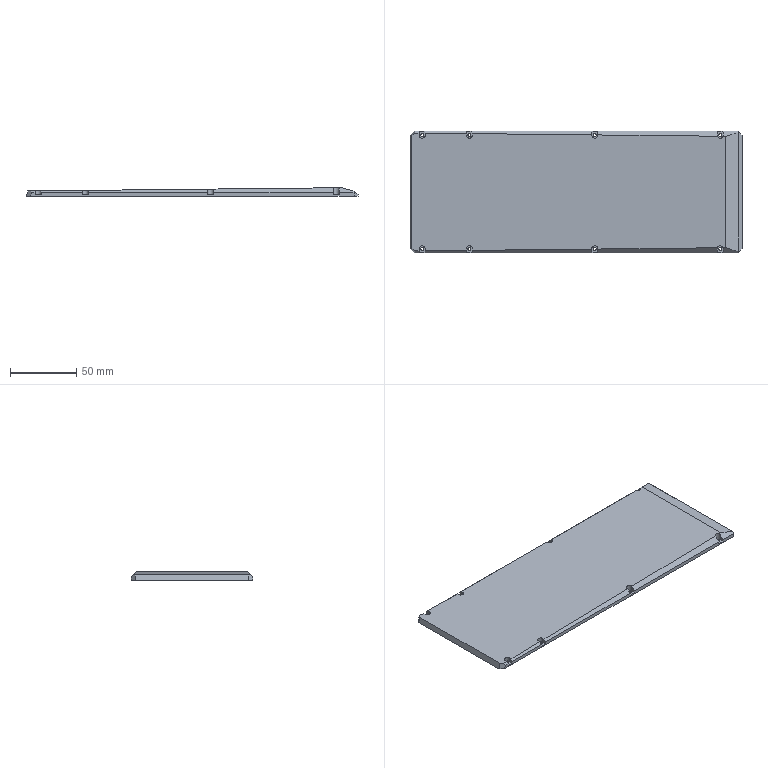Part | 1 solid | 100 faces | box 251.5 x 92 x 6.5 mm | volume 69822 mm3 | plane 62 | cylinder 34 | cone 4 | commonest cylinder face diameters 2.4 x16 6 x10 4.5 x8